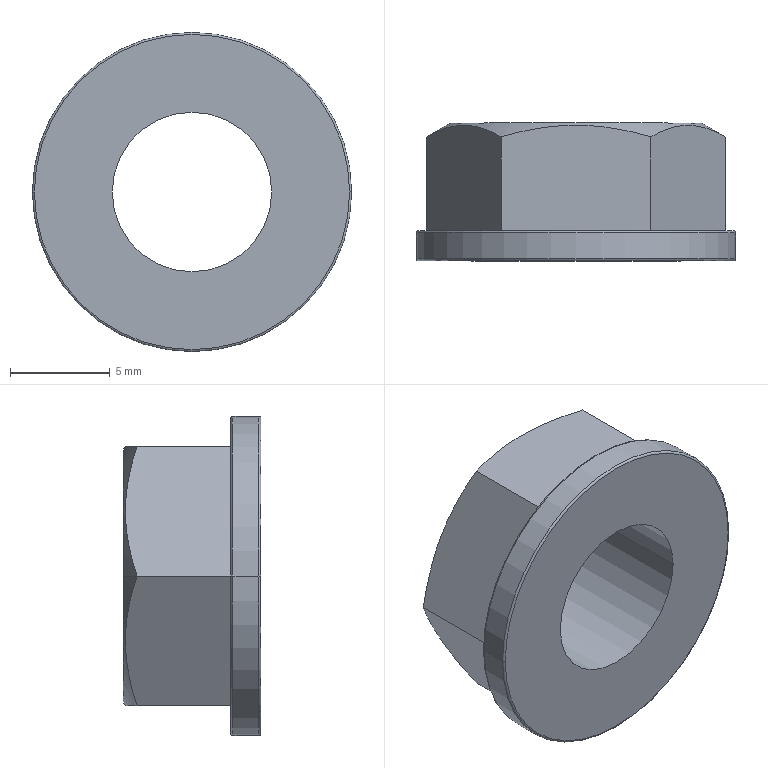Part | STEP file | LIB_68452121_M8_SERPRESS | 1 solid | 19 faces | box 16 x 6.9 x 16 mm | volume 740.456 mm3 | plane 9 | cylinder 4 | torus 4 | cone 2 | commonest cylinder face diameters 8 x2 16 x2